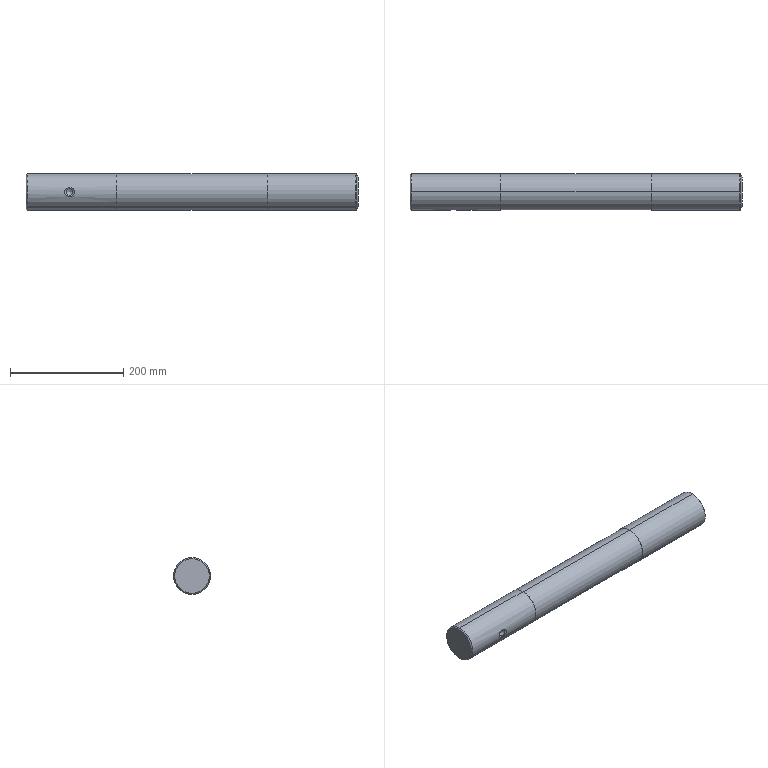Part | SolidWorks | features Chamfer 2, Fillet 1, HoleWzd 1, Revolution 1 | 1 solid | 24 faces | box 586 x 65 x 65 mm | volume 1913862 mm3 | cylinder 8 | cone 8 | torus 4 | plane 4 | commonest cylinder face diameters 65 x4 12 x2 64 x2
STEP:
#1=CARTESIAN_POINT('',(77.,-22.5,6.));
#2=VERTEX_POINT('',#1);
#3=CARTESIAN_POINT('',(77.,-22.5,-6.));
#4=VERTEX_POINT('',#3);
#5=CARTESIAN_POINT('',(77.,-22.5,0.));
#6=DIRECTION('',(0.,-1.,0.));
#7=DIRECTION('',(0.,0.,-1.));
#8=AXIS2_PLACEMENT_3D('',#5,#6,#7);
#9=CIRCLE('',#8,6.);
#10=EDGE_CURVE('',#2,#4,#9,.T.);
#11=ORIENTED_EDGE('',*,*,#10,.F.);
#12=CARTESIAN_POINT('',(77.,-30.768,6.));
#13=VERTEX_POINT('',#12);
#14=CARTESIAN_POINT('',(77.,-32.5,6.));
#15=DIRECTION('',(0.,-1.,0.));
#16=VECTOR('',#15,1000.);
#17=LINE('',#14,#16);
#18=EDGE_CURVE('',#2,#13,#17,.T.);
#19=ORIENTED_EDGE('',*,*,#18,.T.);
#20=CARTESIAN_POINT('',(77.,-30.768,-6.));
#21=VERTEX_POINT('',#20);
#22=CARTESIAN_POINT('',(77.,-30.768,0.));
#23=DIRECTION('',(0.,-1.,0.));
#24=DIRECTION('',(0.,0.,-1.));
#25=AXIS2_PLACEMENT_3D('',#22,#23,#24);
#26=CIRCLE('',#25,6.);
#27=EDGE_CURVE('',#13,#21,#26,.T.);
#28=ORIENTED_EDGE('',*,*,#27,.T.);
#29=CARTESIAN_POINT('',(77.,-32.5,-6.));
#30=DIRECTION('',(0.,-1.,0.));
#31=VECTOR('',#30,1000.);
#32=LINE('',#29,#31);
#33=EDGE_CURVE('',#4,#21,#32,.T.);
#34=ORIENTED_EDGE('',*,*,#33,.F.);
#35=EDGE_LOOP('',(#11,#19,#28,#34));
#36=FACE_OUTER_BOUND('',#35,.T.);
#37=CARTESIAN_POINT('',(77.,-32.5,0.));
#38=DIRECTION('',(0.,-1.,0.));
#39=DIRECTION('',(0.,0.,-1.));
#40=AXIS2_PLACEMENT_3D('',#37,#38,#39);
#41=CYLINDRICAL_SURFACE('',#40,6.);
#42=ADVANCED_FACE('',(#36),#41,.F.);
#43=CARTESIAN_POINT('',(77.,-18.895,0.));
#44=VERTEX_POINT('',#43);
#45=CARTESIAN_POINT('',(77.,-22.5,-6.));
#46=DIRECTION('',(0.,-0.515,-0.8572));
#47=VECTOR('',#46,1000.);
#48=LINE('',#45,#47);
#49=EDGE_CURVE('',#44,#4,#48,.T.);
#50=ORIENTED_EDGE('',*,*,#49,.F.);
#51=CARTESIAN_POINT('',(77.,-22.5,6.));
#52=DIRECTION('',(0.,-0.515,0.8572));
#53=VECTOR('',#52,1000.);
#54=LINE('',#51,#53);
#55=EDGE_CURVE('',#44,#2,#54,.T.);
#56=ORIENTED_EDGE('',*,*,#55,.T.);
#57=ORIENTED_EDGE('',*,*,#10,.T.);
#58=EDGE_LOOP('',(#50,#56,#57));
#59=FACE_OUTER_BOUND('',#58,.T.);
#60=CARTESIAN_POINT('',(77.,-22.5,0.));
#61=DIRECTION('',(0.,-1.,0.));
#62=DIRECTION('',(0.,0.,-1.));
#63=AXIS2_PLACEMENT_3D('',#60,#61,#62);
#64=CONICAL_SURFACE('',#63,6.,1.03);
#65=ADVANCED_FACE('',(#59),#64,.F.);
#66=ORIENTED_EDGE('',*,*,#27,.F.);
#67=CARTESIAN_POINT('',(77.,-31.626,7.486));
#68=VERTEX_POINT('',#67);
#69=CARTESIAN_POINT('',(77.,-32.5,9.));
#70=DIRECTION('',(0.,-0.5,0.866));
#71=VECTOR('',#70,1000.);
#72=LINE('',#69,#71);
#73=EDGE_CURVE('',#13,#68,#72,.T.);
#74=ORIENTED_EDGE('',*,*,#73,.T.);
#75=CARTESIAN_POINT('',(77.,-31.626,-7.486));
#76=VERTEX_POINT('',#75);
#77=CARTESIAN_POINT('',(77.,-31.626,-7.486));
#78=CARTESIAN_POINT('',(76.461,-31.626,-7.486));
#79=CARTESIAN_POINT('',(75.923,-31.636,-7.445));
#80=CARTESIAN_POINT('',(75.117,-31.665,-7.32));
#81=CARTESIAN_POINT('',(74.849,-31.677,-7.268));
#82=CARTESIAN_POINT('',(74.322,-31.705,-7.143));
#83=CARTESIAN_POINT('',(74.063,-31.722,-7.071));
#84=CARTESIAN_POINT('',(73.296,-31.776,-6.824));
#85=CARTESIAN_POINT('',(72.8,-31.82,-6.62));
#86=CARTESIAN_POINT('',(71.838,-31.918,-6.126));
#87=CARTESIAN_POINT('',(71.373,-31.974,-5.834));
#88=CARTESIAN_POINT('',(70.513,-32.086,-5.179));
#89=CARTESIAN_POINT('',(70.119,-32.144,-4.816));
#90=CARTESIAN_POINT('',(69.585,-32.226,-4.216));
#91=CARTESIAN_POINT('',(69.417,-32.253,-4.007));
#92=CARTESIAN_POINT('',(69.103,-32.304,-3.567));
#93=CARTESIAN_POINT('',(68.956,-32.329,-3.337));
#94=CARTESIAN_POINT('',(68.563,-32.397,-2.63));
#95=CARTESIAN_POINT('',(68.357,-32.434,-2.133));
#96=CARTESIAN_POINT('',(68.072,-32.486,-1.079));
#97=CARTESIAN_POINT('',(68.,-32.5,-0.5447));
#98=CARTESIAN_POINT('',(68.,-32.5,0.2645));
#99=CARTESIAN_POINT('',(68.018,-32.497,0.5376));
#100=CARTESIAN_POINT('',(68.09,-32.483,1.077));
#101=CARTESIAN_POINT('',(68.143,-32.473,1.342));
#102=CARTESIAN_POINT('',(68.284,-32.448,1.863));
#103=CARTESIAN_POINT('',(68.37,-32.432,2.119));
#104=CARTESIAN_POINT('',(68.576,-32.395,2.621));
#105=CARTESIAN_POINT('',(68.695,-32.374,2.867));
#106=CARTESIAN_POINT('',(69.089,-32.306,3.574));
#107=CARTESIAN_POINT('',(69.405,-32.254,4.013));
#108=CARTESIAN_POINT('',(70.125,-32.143,4.824));
#109=CARTESIAN_POINT('',(70.522,-32.085,5.187));
#110=CARTESIAN_POINT('',(71.379,-31.973,5.838));
#111=CARTESIAN_POINT('',(71.842,-31.918,6.128));
#112=CARTESIAN_POINT('',(72.799,-31.82,6.619));
#113=CARTESIAN_POINT('',(73.296,-31.776,6.824));
#114=CARTESIAN_POINT('',(74.069,-31.721,7.073));
#115=CARTESIAN_POINT('',(74.332,-31.705,7.146));
#116=CARTESIAN_POINT('',(74.859,-31.677,7.27));
#117=CARTESIAN_POINT('',(75.123,-31.665,7.321));
#118=CARTESIAN_POINT('',(75.921,-31.636,7.445));
#119=CARTESIAN_POINT('',(76.458,-31.626,7.486));
#120=CARTESIAN_POINT('',(77.,-31.626,7.486));
#121=B_SPLINE_CURVE_WITH_KNOTS('',3,(#77,#78,#79,#80,#81,#82,#83,#84,#85,#86,#87,#88,#89,#90,#91,#92,#93,#94,#95,#96,#97,#98,#99,#100,#101,#102,#103,#104,#105,#106,#107,#108,#109,#110,#111,#112,#113,#114,#115,#116,#117,#118,#119,#120),.UNSPECIFIED.,.F.,.F.,(4,2,2,2,2,2,2,2,2,2,2,2,2,2,2,2,2,2,2,2,2,4),(0.04529,0.0469,0.04771,0.04851,0.05013,0.05174,0.05335,0.05416,0.05496,0.05658,0.05819,0.05899,0.0598,0.06061,0.06141,0.06303,0.06464,0.06625,0.06786,0.06867,0.06948,0.07109),.UNSPECIFIED.);
#122=EDGE_CURVE('',#76,#68,#121,.T.);
#123=ORIENTED_EDGE('',*,*,#122,.F.);
#124=CARTESIAN_POINT('',(77.,-32.5,-9.));
#125=DIRECTION('',(0.,-0.5,-0.866));
#126=VECTOR('',#125,1000.);
#127=LINE('',#124,#126);
#128=EDGE_CURVE('',#21,#76,#127,.T.);
#129=ORIENTED_EDGE('',*,*,#128,.F.);
#130=EDGE_LOOP('',(#66,#74,#123,#129));
#131=FACE_OUTER_BOUND('',#130,.T.);
#132=CARTESIAN_POINT('',(77.,-32.5,0.));
#133=DIRECTION('',(0.,-1.,0.));
#134=DIRECTION('',(0.,0.,-1.));
#135=AXIS2_PLACEMENT_3D('',#132,#133,#134);
#136=CONICAL_SURFACE('',#135,9.,1.047);
#137=ADVANCED_FACE('',(#131),#136,.F.);
#138=CARTESIAN_POINT('',(586.,0.,-26.366));
#139=VERTEX_POINT('',#138);
#140=CARTESIAN_POINT('',(586.,0.,26.366));
#141=VERTEX_POINT('',#140);
#142=CARTESIAN_POINT('',(586.,0.,0.));
#143=DIRECTION('',(1.,0.,0.));
#144=DIRECTION('',(0.,0.,1.));
#145=AXIS2_PLACEMENT_3D('',#142,#143,#144);
#146=CIRCLE('',#145,26.366);
#147=EDGE_CURVE('',#139,#141,#146,.T.);
#148=ORIENTED_EDGE('',*,*,#147,.F.);
#149=CARTESIAN_POINT('',(585.933,0.,-26.616));
#150=VERTEX_POINT('',#149);
#151=CARTESIAN_POINT('',(585.5,0.,-26.366));
#152=DIRECTION('',(0.,1.,0.));
#153=DIRECTION('',(0.,0.,1.));
#154=AXIS2_PLACEMENT_3D('',#151,#152,#153);
#155=CIRCLE('',#154,0.5);
#156=EDGE_CURVE('',#139,#150,#155,.T.);
#157=ORIENTED_EDGE('',*,*,#156,.T.);
#158=CARTESIAN_POINT('',(585.933,0.,26.616));
#159=VERTEX_POINT('',#158);
#160=CARTESIAN_POINT('',(585.933,0.,0.));
#161=DIRECTION('',(-1.,0.,0.));
#162=DIRECTION('',(0.,0.,1.));
#163=AXIS2_PLACEMENT_3D('',#160,#161,#162);
#164=CIRCLE('',#163,26.616);
#165=EDGE_CURVE('',#159,#150,#164,.T.);
#166=ORIENTED_EDGE('',*,*,#165,.F.);
#167=CARTESIAN_POINT('',(585.5,0.,26.366));
#168=DIRECTION('',(0.,-1.,0.));
#169=DIRECTION('',(0.,0.,-1.));
#170=AXIS2_PLACEMENT_3D('',#167,#168,#169);
#171=CIRCLE('',#170,0.5);
#172=EDGE_CURVE('',#141,#159,#171,.T.);
#173=ORIENTED_EDGE('',*,*,#172,.F.);
#174=EDGE_LOOP('',(#148,#157,#166,#173));
#175=FACE_OUTER_BOUND('',#174,.T.);
#176=CARTESIAN_POINT('',(585.5,0.,0.));
#177=DIRECTION('',(-1.,0.,0.));
#178=DIRECTION('',(0.,0.,1.));
#179=AXIS2_PLACEMENT_3D('',#176,#177,#178);
#180=TOROIDAL_SURFACE('',#179,26.366,0.5);
#181=ADVANCED_FACE('',(#175),#180,.T.);
#182=CARTESIAN_POINT('',(582.247,0.,32.5));
#183=VERTEX_POINT('',#182);
#184=CARTESIAN_POINT('',(582.247,0.,-32.5));
#185=VERTEX_POINT('',#184);
#186=CARTESIAN_POINT('',(582.247,0.,0.));
#187=DIRECTION('',(-1.,0.,0.));
#188=DIRECTION('',(0.,0.,-1.));
#189=AXIS2_PLACEMENT_3D('',#186,#187,#188);
#190=CIRCLE('',#189,32.5);
#191=EDGE_CURVE('',#183,#185,#190,.T.);
#192=ORIENTED_EDGE('',*,*,#191,.F.);
#193=CARTESIAN_POINT('',(582.68,0.,32.25));
#194=VERTEX_POINT('',#193);
#195=CARTESIAN_POINT('',(582.247,0.,32.));
#196=DIRECTION('',(0.,1.,0.));
#197=DIRECTION('',(0.,0.,1.));
#198=AXIS2_PLACEMENT_3D('',#195,#196,#197);
#199=CIRCLE('',#198,0.5);
#200=EDGE_CURVE('',#183,#194,#199,.T.);
#201=ORIENTED_EDGE('',*,*,#200,.T.);
#202=CARTESIAN_POINT('',(582.68,0.,-32.25));
#203=VERTEX_POINT('',#202);
#204=CARTESIAN_POINT('',(582.68,0.,0.));
#205=DIRECTION('',(1.,0.,0.));
#206=DIRECTION('',(0.,0.,1.));
#207=AXIS2_PLACEMENT_3D('',#204,#205,#206);
#208=CIRCLE('',#207,32.25);
#209=EDGE_CURVE('',#203,#194,#208,.T.);
#210=ORIENTED_EDGE('',*,*,#209,.F.);
#211=CARTESIAN_POINT('',(582.247,0.,-32.));
#212=DIRECTION('',(0.,-1.,0.));
#213=DIRECTION('',(0.,0.,-1.));
#214=AXIS2_PLACEMENT_3D('',#211,#212,#213);
#215=CIRCLE('',#214,0.5);
#216=EDGE_CURVE('',#185,#203,#215,.T.);
#217=ORIENTED_EDGE('',*,*,#216,.F.);
#218=EDGE_LOOP('',(#192,#201,#210,#217));
#219=FACE_OUTER_BOUND('',#218,.T.);
#220=CARTESIAN_POINT('',(582.247,0.,0.));
#221=DIRECTION('',(1.,0.,0.));
#222=DIRECTION('',(0.,0.,-1.));
#223=AXIS2_PLACEMENT_3D('',#220,#221,#222);
#224=TOROIDAL_SURFACE('',#223,32.,0.5);
#225=ADVANCED_FACE('',(#219),#224,.T.);
#226=ORIENTED_EDGE('',*,*,#165,.T.);
#227=CARTESIAN_POINT('',(582.536,0.,-32.5));
#228=DIRECTION('',(-0.5,0.,-0.866));
#229=VECTOR('',#228,1000.);
#230=LINE('',#227,#229);
#231=EDGE_CURVE('',#150,#203,#230,.T.);
#232=ORIENTED_EDGE('',*,*,#231,.T.);
#233=ORIENTED_EDGE('',*,*,#209,.T.);
#234=CARTESIAN_POINT('',(582.536,0.,32.5));
#235=DIRECTION('',(-0.5,0.,0.866));
#236=VECTOR('',#235,1000.);
#237=LINE('',#234,#236);
#238=EDGE_CURVE('',#159,#194,#237,.T.);
#239=ORIENTED_EDGE('',*,*,#238,.F.);
#240=EDGE_LOOP('',(#226,#232,#233,#239));
#241=FACE_OUTER_BOUND('',#240,.T.);
#242=CARTESIAN_POINT('',(582.536,0.,0.));
#243=DIRECTION('',(-1.,0.,0.));
#244=DIRECTION('',(0.,0.,1.));
#245=AXIS2_PLACEMENT_3D('',#242,#243,#244);
#246=CONICAL_SURFACE('',#245,32.5,1.047);
#247=ADVANCED_FACE('',(#241),#246,.T.);
#248=CARTESIAN_POINT('',(0.,0.,30.5));
#249=VERTEX_POINT('',#248);
#250=CARTESIAN_POINT('',(0.,0.,-30.5));
#251=VERTEX_POINT('',#250);
#252=CARTESIAN_POINT('',(0.,0.,0.));
#253=DIRECTION('',(-1.,0.,0.));
#254=DIRECTION('',(0.,0.,-1.));
#255=AXIS2_PLACEMENT_3D('',#252,#253,#254);
#256=CIRCLE('',#255,30.5);
#257=EDGE_CURVE('',#249,#251,#256,.T.);
#258=ORIENTED_EDGE('',*,*,#257,.F.);
#259=CARTESIAN_POINT('',(2.,0.,32.5));
#260=VERTEX_POINT('',#259);
#261=CARTESIAN_POINT('',(0.,0.,30.5));
#262=DIRECTION('',(0.7071,0.,0.7071));
#263=VECTOR('',#262,1000.);
#264=LINE('',#261,#263);
#265=EDGE_CURVE('',#249,#260,#264,.T.);
#266=ORIENTED_EDGE('',*,*,#265,.T.);
#267=CARTESIAN_POINT('',(2.,0.,-32.5));
#268=VERTEX_POINT('',#267);
#269=CARTESIAN_POINT('',(2.,0.,0.));
#270=DIRECTION('',(1.,0.,0.));
#271=DIRECTION('',(0.,0.,-1.));
#272=AXIS2_PLACEMENT_3D('',#269,#270,#271);
#273=CIRCLE('',#272,32.5);
#274=EDGE_CURVE('',#268,#260,#273,.T.);
#275=ORIENTED_EDGE('',*,*,#274,.F.);
#276=CARTESIAN_POINT('',(0.,0.,-30.5));
#277=DIRECTION('',(0.7071,0.,-0.7071));
#278=VECTOR('',#277,1000.);
#279=LINE('',#276,#278);
#280=EDGE_CURVE('',#251,#268,#279,.T.);
#281=ORIENTED_EDGE('',*,*,#280,.F.);
#282=EDGE_LOOP('',(#258,#266,#275,#281));
#283=FACE_OUTER_BOUND('',#282,.T.);
#284=CARTESIAN_POINT('',(0.,0.,0.));
#285=DIRECTION('',(1.,0.,0.));
#286=DIRECTION('',(0.,0.,-1.));
#287=AXIS2_PLACEMENT_3D('',#284,#285,#286);
#288=CONICAL_SURFACE('',#287,30.5,0.7854);
#289=ADVANCED_FACE('',(#283),#288,.T.);
#290=ORIENTED_EDGE('',*,*,#191,.T.);
#291=CARTESIAN_POINT('',(426.,0.,-32.5));
#292=VERTEX_POINT('',#291);
#293=CARTESIAN_POINT('',(-129.316,0.,-32.5));
#294=DIRECTION('',(-1.,0.,0.));
#295=VECTOR('',#294,1000.);
#296=LINE('',#293,#295);
#297=EDGE_CURVE('',#185,#292,#296,.T.);
#298=ORIENTED_EDGE('',*,*,#297,.T.);
#299=CARTESIAN_POINT('',(426.,0.,32.5));
#300=VERTEX_POINT('',#299);
#301=CARTESIAN_POINT('',(426.,0.,0.));
#302=DIRECTION('',(-1.,0.,0.));
#303=DIRECTION('',(0.,0.,1.));
#304=AXIS2_PLACEMENT_3D('',#301,#302,#303);
#305=CIRCLE('',#304,32.5);
#306=EDGE_CURVE('',#300,#292,#305,.T.);
#307=ORIENTED_EDGE('',*,*,#306,.F.);
#308=CARTESIAN_POINT('',(-129.316,0.,32.5));
#309=DIRECTION('',(-1.,0.,0.));
#310=VECTOR('',#309,1000.);
#311=LINE('',#308,#310);
#312=EDGE_CURVE('',#183,#300,#311,.T.);
#313=ORIENTED_EDGE('',*,*,#312,.F.);
#314=EDGE_LOOP('',(#290,#298,#307,#313));
#315=FACE_OUTER_BOUND('',#314,.T.);
#316=CARTESIAN_POINT('',(-129.316,0.,0.));
#317=DIRECTION('',(-1.,0.,0.));
#318=DIRECTION('',(0.,0.,1.));
#319=AXIS2_PLACEMENT_3D('',#316,#317,#318);
#320=CYLINDRICAL_SURFACE('',#319,32.5);
#321=ADVANCED_FACE('',(#315),#320,.T.);
#322=CARTESIAN_POINT('',(426.,0.,32.));
#323=VERTEX_POINT('',#322);
#324=CARTESIAN_POINT('',(426.,0.,-32.));
#325=VERTEX_POINT('',#324);
#326=CARTESIAN_POINT('',(426.,0.,0.));
#327=DIRECTION('',(-1.,0.,0.));
#328=DIRECTION('',(0.,0.,1.));
#329=AXIS2_PLACEMENT_3D('',#326,#327,#328);
#330=CIRCLE('',#329,32.);
#331=EDGE_CURVE('',#323,#325,#330,.T.);
#332=ORIENTED_EDGE('',*,*,#331,.T.);
#333=CARTESIAN_POINT('',(160.,0.,-32.));
#334=VERTEX_POINT('',#333);
#335=CARTESIAN_POINT('',(-129.316,0.,-32.));
#336=DIRECTION('',(-1.,0.,0.));
#337=VECTOR('',#336,1000.);
#338=LINE('',#335,#337);
#339=EDGE_CURVE('',#325,#334,#338,.T.);
#340=ORIENTED_EDGE('',*,*,#339,.T.);
#341=CARTESIAN_POINT('',(160.,0.,32.));
#342=VERTEX_POINT('',#341);
#343=CARTESIAN_POINT('',(160.,0.,0.));
#344=DIRECTION('',(-1.,0.,0.));
#345=DIRECTION('',(0.,0.,1.));
#346=AXIS2_PLACEMENT_3D('',#343,#344,#345);
#347=CIRCLE('',#346,32.);
#348=EDGE_CURVE('',#342,#334,#347,.T.);
#349=ORIENTED_EDGE('',*,*,#348,.F.);
#350=CARTESIAN_POINT('',(-129.316,0.,32.));
#351=DIRECTION('',(-1.,0.,0.));
#352=VECTOR('',#351,1000.);
#353=LINE('',#350,#352);
#354=EDGE_CURVE('',#323,#342,#353,.T.);
#355=ORIENTED_EDGE('',*,*,#354,.F.);
#356=EDGE_LOOP('',(#332,#340,#349,#355));
#357=FACE_OUTER_BOUND('',#356,.T.);
#358=CARTESIAN_POINT('',(-129.316,0.,0.));
#359=DIRECTION('',(-1.,0.,0.));
#360=DIRECTION('',(0.,0.,1.));
#361=AXIS2_PLACEMENT_3D('',#358,#359,#360);
#362=CYLINDRICAL_SURFACE('',#361,32.);
#363=ADVANCED_FACE('',(#357),#362,.T.);
#364=CARTESIAN_POINT('',(160.,0.,32.5));
#365=VERTEX_POINT('',#364);
#366=CARTESIAN_POINT('',(160.,0.,-32.5));
#367=VERTEX_POINT('',#366);
#368=CARTESIAN_POINT('',(160.,0.,0.));
#369=DIRECTION('',(-1.,0.,0.));
#370=DIRECTION('',(0.,0.,1.));
#371=AXIS2_PLACEMENT_3D('',#368,#369,#370);
#372=CIRCLE('',#371,32.5);
#373=EDGE_CURVE('',#365,#367,#372,.T.);
#374=ORIENTED_EDGE('',*,*,#373,.T.);
#375=CARTESIAN_POINT('',(-129.316,0.,-32.5));
#376=DIRECTION('',(-1.,0.,0.));
#377=VECTOR('',#376,1000.);
#378=LINE('',#375,#377);
#379=EDGE_CURVE('',#367,#268,#378,.T.);
#380=ORIENTED_EDGE('',*,*,#379,.T.);
#381=ORIENTED_EDGE('',*,*,#274,.T.);
#382=CARTESIAN_POINT('',(-129.316,0.,32.5));
#383=DIRECTION('',(-1.,0.,0.));
#384=VECTOR('',#383,1000.);
#385=LINE('',#382,#384);
#386=EDGE_CURVE('',#365,#260,#385,.T.);
#387=ORIENTED_EDGE('',*,*,#386,.F.);
#388=EDGE_LOOP('',(#374,#380,#381,#387));
#389=FACE_OUTER_BOUND('',#388,.T.);
#390=CARTESIAN_POINT('',(-129.316,0.,0.));
#391=DIRECTION('',(-1.,0.,0.));
#392=DIRECTION('',(0.,0.,1.));
#393=AXIS2_PLACEMENT_3D('',#390,#391,#392);
#394=CYLINDRICAL_SURFACE('',#393,32.5);
#395=ADVANCED_FACE('',(#389),#394,.T.);
#396=CARTESIAN_POINT('',(0.,0.,0.));
#397=DIRECTION('',(-1.,0.,0.));
#398=DIRECTION('',(0.,0.,-1.));
#399=AXIS2_PLACEMENT_3D('',#396,#397,#398);
#400=CIRCLE('',#399,30.5);
#401=EDGE_CURVE('',#251,#249,#400,.T.);
#402=ORIENTED_EDGE('',*,*,#401,.T.);
#403=ORIENTED_EDGE('',*,*,#257,.T.);
#404=EDGE_LOOP('',(#402,#403));
#405=FACE_OUTER_BOUND('',#404,.T.);
#406=CARTESIAN_POINT('',(0.,0.,0.));
#407=DIRECTION('',(1.,0.,0.));
#408=DIRECTION('',(0.,0.,-1.));
#409=AXIS2_PLACEMENT_3D('',#406,#407,#408);
#410=PLANE('',#409);
#411=ADVANCED_FACE('',(#405),#410,.F.);
#412=ORIENTED_EDGE('',*,*,#379,.F.);
#413=CARTESIAN_POINT('',(160.,0.,0.));
#414=DIRECTION('',(-1.,0.,0.));
#415=DIRECTION('',(0.,0.,1.));
#416=AXIS2_PLACEMENT_3D('',#413,#414,#415);
#417=CIRCLE('',#416,32.5);
#418=EDGE_CURVE('',#367,#365,#417,.T.);
#419=ORIENTED_EDGE('',*,*,#418,.T.);
#420=ORIENTED_EDGE('',*,*,#386,.T.);
#421=CARTESIAN_POINT('',(2.,0.,0.));
#422=DIRECTION('',(1.,0.,0.));
#423=DIRECTION('',(0.,0.,-1.));
#424=AXIS2_PLACEMENT_3D('',#421,#422,#423);
#425=CIRCLE('',#424,32.5);
#426=EDGE_CURVE('',#260,#268,#425,.T.);
#427=ORIENTED_EDGE('',*,*,#426,.T.);
#428=EDGE_LOOP('',(#412,#419,#420,#427));
#429=FACE_OUTER_BOUND('',#428,.T.);
#430=ORIENTED_EDGE('',*,*,#122,.T.);
#431=CARTESIAN_POINT('',(77.,-31.626,7.486));
#432=CARTESIAN_POINT('',(77.271,-31.626,7.486));
#433=CARTESIAN_POINT('',(77.544,-31.629,7.476));
#434=CARTESIAN_POINT('',(78.084,-31.638,7.434));
#435=CARTESIAN_POINT('',(78.352,-31.646,7.403));
#436=CARTESIAN_POINT('',(79.148,-31.675,7.279));
#437=CARTESIAN_POINT('',(79.67,-31.703,7.156));
#438=CARTESIAN_POINT('',(80.441,-31.757,6.909));
#439=CARTESIAN_POINT('',(80.696,-31.778,6.816));
#440=CARTESIAN_POINT('',(81.196,-31.821,6.609));
#441=CARTESIAN_POINT('',(81.441,-31.844,6.496));
#442=CARTESIAN_POINT('',(82.155,-31.918,6.129));
#443=CARTESIAN_POINT('',(82.608,-31.971,5.847));
#444=CARTESIAN_POINT('',(83.462,-32.083,5.2));
#445=CARTESIAN_POINT('',(83.867,-32.142,4.831));
#446=CARTESIAN_POINT('',(84.582,-32.252,4.029));
#447=CARTESIAN_POINT('',(84.898,-32.304,3.595));
#448=CARTESIAN_POINT('',(85.43,-32.396,2.646));
#449=CARTESIAN_POINT('',(85.637,-32.433,2.147));
#450=CARTESIAN_POINT('',(85.85,-32.472,1.371));
#451=CARTESIAN_POINT('',(85.905,-32.482,1.107));
#452=CARTESIAN_POINT('',(85.98,-32.496,0.5677));
#453=CARTESIAN_POINT('',(85.999,-32.5,0.2938));
#454=CARTESIAN_POINT('',(86.002,-32.5,-0.5173));
#455=CARTESIAN_POINT('',(85.932,-32.487,-1.055));
#456=CARTESIAN_POINT('',(85.651,-32.436,-2.111));
#457=CARTESIAN_POINT('',(85.446,-32.399,-2.61));
#458=CARTESIAN_POINT('',(85.052,-32.331,-3.322));
#459=CARTESIAN_POINT('',(84.906,-32.306,-3.553));
#460=CARTESIAN_POINT('',(84.593,-32.254,-3.994));
#461=CARTESIAN_POINT('',(84.425,-32.228,-4.204));
#462=CARTESIAN_POINT('',(83.889,-32.145,-4.809));
#463=CARTESIAN_POINT('',(83.486,-32.086,-5.18));
#464=CARTESIAN_POINT('',(82.629,-31.974,-5.833));
#465=CARTESIAN_POINT('',(82.173,-31.92,-6.119));
#466=CARTESIAN_POINT('',(81.45,-31.845,-6.492));
#467=CARTESIAN_POINT('',(81.203,-31.822,-6.606));
#468=CARTESIAN_POINT('',(80.703,-31.778,-6.813));
#469=CARTESIAN_POINT('',(80.45,-31.758,-6.905));
#470=CARTESIAN_POINT('',(79.681,-31.703,-7.153));
#471=CARTESIAN_POINT('',(79.156,-31.675,-7.278));
#472=CARTESIAN_POINT('',(78.079,-31.636,-7.445));
#473=CARTESIAN_POINT('',(77.539,-31.626,-7.486));
#474=CARTESIAN_POINT('',(77.,-31.626,-7.486));
#475=B_SPLINE_CURVE_WITH_KNOTS('',3,(#431,#432,#433,#434,#435,#436,#437,#438,#439,#440,#441,#442,#443,#444,#445,#446,#447,#448,#449,#450,#451,#452,#453,#454,#455,#456,#457,#458,#459,#460,#461,#462,#463,#464,#465,#466,#467,#468,#469,#470,#471,#472,#473,#474),.UNSPECIFIED.,.F.,.F.,(4,2,2,2,2,2,2,2,2,2,2,2,2,2,2,2,2,2,2,2,2,4),(0.0195,0.0203,0.02111,0.02272,0.02353,0.02433,0.02595,0.02756,0.02917,0.03078,0.03159,0.03239,0.034,0.03562,0.03642,0.03723,0.03884,0.04045,0.04126,0.04206,0.04368,0.04529),.UNSPECIFIED.);
#476=EDGE_CURVE('',#68,#76,#475,.T.);
#477=ORIENTED_EDGE('',*,*,#476,.T.);
#478=EDGE_LOOP('',(#430,#477));
#479=FACE_BOUND('',#478,.T.);
#480=CARTESIAN_POINT('',(-129.316,0.,0.));
#481=DIRECTION('',(-1.,0.,0.));
#482=DIRECTION('',(0.,0.,1.));
#483=AXIS2_PLACEMENT_3D('',#480,#481,#482);
#484=CYLINDRICAL_SURFACE('',#483,32.5);
#485=ADVANCED_FACE('',(#429,#479),#484,.T.);
#486=ORIENTED_EDGE('',*,*,#373,.F.);
#487=ORIENTED_EDGE('',*,*,#418,.F.);
#488=EDGE_LOOP('',(#486,#487));
#489=FACE_OUTER_BOUND('',#488,.T.);
#490=ORIENTED_EDGE('',*,*,#348,.T.);
#491=CARTESIAN_POINT('',(160.,0.,0.));
#492=DIRECTION('',(-1.,0.,0.));
#493=DIRECTION('',(0.,0.,1.));
#494=AXIS2_PLACEMENT_3D('',#491,#492,#493);
#495=CIRCLE('',#494,32.);
#496=EDGE_CURVE('',#334,#342,#495,.T.);
#497=ORIENTED_EDGE('',*,*,#496,.T.);
#498=EDGE_LOOP('',(#490,#497));
#499=FACE_BOUND('',#498,.T.);
#500=CARTESIAN_POINT('',(160.,32.5,0.));
#501=DIRECTION('',(-1.,0.,0.));
#502=DIRECTION('',(0.,0.,1.));
#503=AXIS2_PLACEMENT_3D('',#500,#501,#502);
#504=PLANE('',#503);
#505=ADVANCED_FACE('',(#489,#499),#504,.F.);
#506=ORIENTED_EDGE('',*,*,#339,.F.);
#507=CARTESIAN_POINT('',(426.,0.,0.));
#508=DIRECTION('',(-1.,0.,0.));
#509=DIRECTION('',(0.,0.,1.));
#510=AXIS2_PLACEMENT_3D('',#507,#508,#509);
#511=CIRCLE('',#510,32.);
#512=EDGE_CURVE('',#325,#323,#511,.T.);
#513=ORIENTED_EDGE('',*,*,#512,.T.);
#514=ORIENTED_EDGE('',*,*,#354,.T.);
#515=ORIENTED_EDGE('',*,*,#496,.F.);
#516=EDGE_LOOP('',(#506,#513,#514,#515));
#517=FACE_OUTER_BOUND('',#516,.T.);
#518=CARTESIAN_POINT('',(-129.316,0.,0.));
#519=DIRECTION('',(-1.,0.,0.));
#520=DIRECTION('',(0.,0.,1.));
#521=AXIS2_PLACEMENT_3D('',#518,#519,#520);
#522=CYLINDRICAL_SURFACE('',#521,32.);
#523=ADVANCED_FACE('',(#517),#522,.T.);
#524=ORIENTED_EDGE('',*,*,#331,.F.);
#525=ORIENTED_EDGE('',*,*,#512,.F.);
#526=EDGE_LOOP('',(#524,#525));
#527=FACE_BOUND('',#526,.T.);
#528=ORIENTED_EDGE('',*,*,#306,.T.);
#529=CARTESIAN_POINT('',(426.,0.,0.));
#530=DIRECTION('',(-1.,0.,0.));
#531=DIRECTION('',(0.,0.,1.));
#532=AXIS2_PLACEMENT_3D('',#529,#530,#531);
#533=CIRCLE('',#532,32.5);
#534=EDGE_CURVE('',#292,#300,#533,.T.);
#535=ORIENTED_EDGE('',*,*,#534,.T.);
#536=EDGE_LOOP('',(#528,#535));
#537=FACE_OUTER_BOUND('',#536,.T.);
#538=CARTESIAN_POINT('',(426.,32.,0.));
#539=DIRECTION('',(1.,0.,0.));
#540=DIRECTION('',(0.,0.,-1.));
#541=AXIS2_PLACEMENT_3D('',#538,#539,#540);
#542=PLANE('',#541);
#543=ADVANCED_FACE('',(#527,#537),#542,.F.);
#544=ORIENTED_EDGE('',*,*,#297,.F.);
#545=CARTESIAN_POINT('',(582.247,0.,0.));
#546=DIRECTION('',(-1.,0.,0.));
#547=DIRECTION('',(0.,0.,-1.));
#548=AXIS2_PLACEMENT_3D('',#545,#546,#547);
#549=CIRCLE('',#548,32.5);
#550=EDGE_CURVE('',#185,#183,#549,.T.);
#551=ORIENTED_EDGE('',*,*,#550,.T.);
#552=ORIENTED_EDGE('',*,*,#312,.T.);
#553=ORIENTED_EDGE('',*,*,#534,.F.);
#554=EDGE_LOOP('',(#544,#551,#552,#553));
#555=FACE_OUTER_BOUND('',#554,.T.);
#556=CARTESIAN_POINT('',(-129.316,0.,0.));
#557=DIRECTION('',(-1.,0.,0.));
#558=DIRECTION('',(0.,0.,1.));
#559=AXIS2_PLACEMENT_3D('',#556,#557,#558);
#560=CYLINDRICAL_SURFACE('',#559,32.5);
#561=ADVANCED_FACE('',(#555),#560,.T.);
#562=CARTESIAN_POINT('',(586.,0.,0.));
#563=DIRECTION('',(1.,0.,0.));
#564=DIRECTION('',(0.,0.,1.));
#565=AXIS2_PLACEMENT_3D('',#562,#563,#564);
#566=CIRCLE('',#565,26.366);
#567=EDGE_CURVE('',#141,#139,#566,.T.);
#568=ORIENTED_EDGE('',*,*,#567,.T.);
#569=ORIENTED_EDGE('',*,*,#147,.T.);
#570=EDGE_LOOP('',(#568,#569));
#571=FACE_OUTER_BOUND('',#570,.T.);
#572=CARTESIAN_POINT('',(586.,32.5,0.));
#573=DIRECTION('',(-1.,0.,0.));
#574=DIRECTION('',(0.,0.,1.));
#575=AXIS2_PLACEMENT_3D('',#572,#573,#574);
#576=PLANE('',#575);
#577=ADVANCED_FACE('',(#571),#576,.F.);
#578=ORIENTED_EDGE('',*,*,#265,.F.);
#579=ORIENTED_EDGE('',*,*,#401,.F.);
#580=ORIENTED_EDGE('',*,*,#280,.T.);
#581=ORIENTED_EDGE('',*,*,#426,.F.);
#582=EDGE_LOOP('',(#578,#579,#580,#581));
#583=FACE_OUTER_BOUND('',#582,.T.);
#584=CARTESIAN_POINT('',(0.,0.,0.));
#585=DIRECTION('',(1.,0.,0.));
#586=DIRECTION('',(0.,0.,-1.));
#587=AXIS2_PLACEMENT_3D('',#584,#585,#586);
#588=CONICAL_SURFACE('',#587,30.5,0.7854);
#589=ADVANCED_FACE('',(#583),#588,.T.);
#590=ORIENTED_EDGE('',*,*,#231,.F.);
#591=CARTESIAN_POINT('',(585.933,0.,0.));
#592=DIRECTION('',(-1.,0.,0.));
#593=DIRECTION('',(0.,0.,1.));
#594=AXIS2_PLACEMENT_3D('',#591,#592,#593);
#595=CIRCLE('',#594,26.616);
#596=EDGE_CURVE('',#150,#159,#595,.T.);
#597=ORIENTED_EDGE('',*,*,#596,.T.);
#598=ORIENTED_EDGE('',*,*,#238,.T.);
#599=CARTESIAN_POINT('',(582.68,0.,0.));
#600=DIRECTION('',(1.,0.,0.));
#601=DIRECTION('',(0.,0.,1.));
#602=AXIS2_PLACEMENT_3D('',#599,#600,#601);
#603=CIRCLE('',#602,32.25);
#604=EDGE_CURVE('',#194,#203,#603,.T.);
#605=ORIENTED_EDGE('',*,*,#604,.T.);
#606=EDGE_LOOP('',(#590,#597,#598,#605));
#607=FACE_OUTER_BOUND('',#606,.T.);
#608=CARTESIAN_POINT('',(582.536,0.,0.));
#609=DIRECTION('',(-1.,0.,0.));
#610=DIRECTION('',(0.,0.,1.));
#611=AXIS2_PLACEMENT_3D('',#608,#609,#610);
#612=CONICAL_SURFACE('',#611,32.5,1.047);
#613=ADVANCED_FACE('',(#607),#612,.T.);
#614=ORIENTED_EDGE('',*,*,#200,.F.);
#615=ORIENTED_EDGE('',*,*,#550,.F.);
#616=ORIENTED_EDGE('',*,*,#216,.T.);
#617=ORIENTED_EDGE('',*,*,#604,.F.);
#618=EDGE_LOOP('',(#614,#615,#616,#617));
#619=FACE_OUTER_BOUND('',#618,.T.);
#620=CARTESIAN_POINT('',(582.247,0.,0.));
#621=DIRECTION('',(1.,0.,0.));
#622=DIRECTION('',(0.,0.,-1.));
#623=AXIS2_PLACEMENT_3D('',#620,#621,#622);
#624=TOROIDAL_SURFACE('',#623,32.,0.5);
#625=ADVANCED_FACE('',(#619),#624,.T.);
#626=ORIENTED_EDGE('',*,*,#156,.F.);
#627=ORIENTED_EDGE('',*,*,#567,.F.);
#628=ORIENTED_EDGE('',*,*,#172,.T.);
#629=ORIENTED_EDGE('',*,*,#596,.F.);
#630=EDGE_LOOP('',(#626,#627,#628,#629));
#631=FACE_OUTER_BOUND('',#630,.T.);
#632=CARTESIAN_POINT('',(585.5,0.,0.));
#633=DIRECTION('',(-1.,0.,0.));
#634=DIRECTION('',(0.,0.,1.));
#635=AXIS2_PLACEMENT_3D('',#632,#633,#634);
#636=TOROIDAL_SURFACE('',#635,26.366,0.5);
#637=ADVANCED_FACE('',(#631),#636,.T.);
#638=ORIENTED_EDGE('',*,*,#73,.F.);
#639=CARTESIAN_POINT('',(77.,-30.768,0.));
#640=DIRECTION('',(0.,-1.,0.));
#641=DIRECTION('',(0.,0.,-1.));
#642=AXIS2_PLACEMENT_3D('',#639,#640,#641);
#643=CIRCLE('',#642,6.);
#644=EDGE_CURVE('',#21,#13,#643,.T.);
#645=ORIENTED_EDGE('',*,*,#644,.F.);
#646=ORIENTED_EDGE('',*,*,#128,.T.);
#647=ORIENTED_EDGE('',*,*,#476,.F.);
#648=EDGE_LOOP('',(#638,#645,#646,#647));
#649=FACE_OUTER_BOUND('',#648,.T.);
#650=CARTESIAN_POINT('',(77.,-32.5,0.));
#651=DIRECTION('',(0.,-1.,0.));
#652=DIRECTION('',(0.,0.,-1.));
#653=AXIS2_PLACEMENT_3D('',#650,#651,#652);
#654=CONICAL_SURFACE('',#653,9.,1.047);
#655=ADVANCED_FACE('',(#649),#654,.F.);
#656=ORIENTED_EDGE('',*,*,#55,.F.);
#657=ORIENTED_EDGE('',*,*,#49,.T.);
#658=CARTESIAN_POINT('',(77.,-22.5,0.));
#659=DIRECTION('',(0.,-1.,0.));
#660=DIRECTION('',(0.,0.,-1.));
#661=AXIS2_PLACEMENT_3D('',#658,#659,#660);
#662=CIRCLE('',#661,6.);
#663=EDGE_CURVE('',#4,#2,#662,.T.);
#664=ORIENTED_EDGE('',*,*,#663,.T.);
#665=EDGE_LOOP('',(#656,#657,#664));
#666=FACE_OUTER_BOUND('',#665,.T.);
#667=CARTESIAN_POINT('',(77.,-22.5,0.));
#668=DIRECTION('',(0.,-1.,0.));
#669=DIRECTION('',(0.,0.,-1.));
#670=AXIS2_PLACEMENT_3D('',#667,#668,#669);
#671=CONICAL_SURFACE('',#670,6.,1.03);
#672=ADVANCED_FACE('',(#666),#671,.F.);
#673=ORIENTED_EDGE('',*,*,#18,.F.);
#674=ORIENTED_EDGE('',*,*,#663,.F.);
#675=ORIENTED_EDGE('',*,*,#33,.T.);
#676=ORIENTED_EDGE('',*,*,#644,.T.);
#677=EDGE_LOOP('',(#673,#674,#675,#676));
#678=FACE_OUTER_BOUND('',#677,.T.);
#679=CARTESIAN_POINT('',(77.,-32.5,0.));
#680=DIRECTION('',(0.,-1.,0.));
#681=DIRECTION('',(0.,0.,-1.));
#682=AXIS2_PLACEMENT_3D('',#679,#680,#681);
#683=CYLINDRICAL_SURFACE('',#682,6.);
#684=ADVANCED_FACE('',(#678),#683,.F.);
#685=CLOSED_SHELL('',(#42,#65,#137,#181,#225,#247,#289,#321,#363,#395,#411,#485,#505,#523,#543,#561,#577,#589,#613,#625,#637,#655,#672,#684));
#686=MANIFOLD_SOLID_BREP('',#685);
#687=CARTESIAN_POINT('',(0.,0.,0.));
#688=DIRECTION('',(0.,0.,1.));
#689=DIRECTION('',(1.,0.,0.));
#690=AXIS2_PLACEMENT_3D('',#687,#688,#689);
#691=(LENGTH_UNIT()NAMED_UNIT(*)SI_UNIT(.MILLI.,.METRE.));
#692=UNCERTAINTY_MEASURE_WITH_UNIT(LENGTH_MEASURE(0.00001),#691,'','');
#693=(NAMED_UNIT(*)PLANE_ANGLE_UNIT()SI_UNIT($,.RADIAN.));
#694=(NAMED_UNIT(*)SI_UNIT($,.STERADIAN.)SOLID_ANGLE_UNIT());
#695=(GEOMETRIC_REPRESENTATION_CONTEXT(3)GLOBAL_UNCERTAINTY_ASSIGNED_CONTEXT((#692))GLOBAL_UNIT_ASSIGNED_CONTEXT((#691,#693,#694))REPRESENTATION_CONTEXT('',''));
#696=ADVANCED_BREP_SHAPE_REPRESENTATION('',(#686,#690),#695);